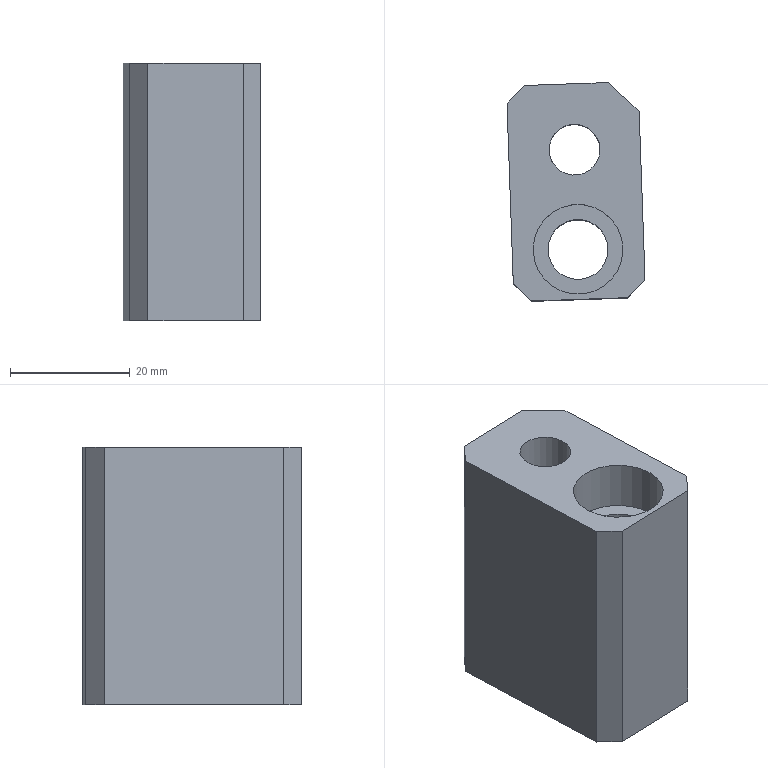Part | NX | features PH-10 2 | 1 solid | 16 faces | box 23.033 x 36.467 x 43 mm | volume 25123 mm3 | plane 12 | cylinder 4 | commonest cylinder face diameters 8.5 x1 10.001 x1 14.5 x1 15 x1
STEP:
#1=CARTESIAN_POINT('',(3339.766,-809.537,945.716));
#2=VERTEX_POINT('',#1);
#3=CARTESIAN_POINT('',(3332.266,-809.537,945.716));
#4=DIRECTION('',(0.,0.,1.));
#5=DIRECTION('',(1.,0.,0.));
#6=AXIS2_PLACEMENT_3D('',#3,#4,#5);
#7=CIRCLE('',#6,7.5);
#8=EDGE_CURVE('',#2,#2,#7,.F.);
#9=ORIENTED_EDGE('',*,*,#8,.T.);
#10=EDGE_LOOP('',(#9));
#11=FACE_BOUND('',#10,.T.);
#12=CARTESIAN_POINT('',(3335.932,-792.749,945.716));
#13=VERTEX_POINT('',#12);
#14=CARTESIAN_POINT('',(3331.685,-792.898,945.716));
#15=DIRECTION('',(0.,0.,1.));
#16=DIRECTION('',(0.9994,0.0349,0.));
#17=AXIS2_PLACEMENT_3D('',#14,#15,#16);
#18=CIRCLE('',#17,4.25);
#19=EDGE_CURVE('',#13,#13,#18,.T.);
#20=ORIENTED_EDGE('',*,*,#19,.F.);
#21=EDGE_LOOP('',(#20));
#22=FACE_BOUND('',#21,.T.);
#23=CARTESIAN_POINT('',(3342.469,-786.517,945.716));
#24=VERTEX_POINT('',#23);
#25=CARTESIAN_POINT('',(3343.446,-814.5,945.716));
#26=VERTEX_POINT('',#25);
#27=CARTESIAN_POINT('',(3342.922,-799.509,945.716));
#28=DIRECTION('',(0.0349,-0.9994,0.));
#29=VECTOR('',#28,1000.);
#30=LINE('',#27,#29);
#31=EDGE_CURVE('',#24,#26,#30,.T.);
#32=ORIENTED_EDGE('',*,*,#31,.F.);
#33=CARTESIAN_POINT('',(3337.297,-781.695,945.716));
#34=VERTEX_POINT('',#33);
#35=CARTESIAN_POINT('',(3343.503,-787.482,945.716));
#36=DIRECTION('',(0.7314,-0.682,0.));
#37=VECTOR('',#36,1000.);
#38=LINE('',#35,#37);
#39=EDGE_CURVE('',#24,#34,#38,.F.);
#40=ORIENTED_EDGE('',*,*,#39,.T.);
#41=CARTESIAN_POINT('',(3323.306,-782.183,945.716));
#42=VERTEX_POINT('',#41);
#43=CARTESIAN_POINT('',(3331.301,-781.904,945.716));
#44=DIRECTION('',(0.9994,0.0349,0.));
#45=VECTOR('',#44,1000.);
#46=LINE('',#43,#45);
#47=EDGE_CURVE('',#42,#34,#46,.T.);
#48=ORIENTED_EDGE('',*,*,#47,.F.);
#49=CARTESIAN_POINT('',(3320.412,-785.286,945.716));
#50=VERTEX_POINT('',#49);
#51=CARTESIAN_POINT('',(3318.483,-787.355,945.716));
#52=DIRECTION('',(0.682,0.7314,0.));
#53=VECTOR('',#52,1000.);
#54=LINE('',#51,#53);
#55=EDGE_CURVE('',#42,#50,#54,.F.);
#56=ORIENTED_EDGE('',*,*,#55,.T.);
#57=CARTESIAN_POINT('',(3321.459,-815.268,945.716));
#58=VERTEX_POINT('',#57);
#59=CARTESIAN_POINT('',(3320.936,-800.277,945.716));
#60=DIRECTION('',(-0.0349,0.9994,0.));
#61=VECTOR('',#60,1000.);
#62=LINE('',#59,#61);
#63=EDGE_CURVE('',#58,#50,#62,.T.);
#64=ORIENTED_EDGE('',*,*,#63,.F.);
#65=CARTESIAN_POINT('',(3324.562,-818.161,945.716));
#66=VERTEX_POINT('',#65);
#67=CARTESIAN_POINT('',(3319.39,-813.339,945.716));
#68=DIRECTION('',(-0.7314,0.682,0.));
#69=VECTOR('',#68,1000.);
#70=LINE('',#67,#69);
#71=EDGE_CURVE('',#58,#66,#70,.F.);
#72=ORIENTED_EDGE('',*,*,#71,.T.);
#73=CARTESIAN_POINT('',(3340.552,-817.603,945.716));
#74=VERTEX_POINT('',#73);
#75=CARTESIAN_POINT('',(3332.557,-817.882,945.716));
#76=DIRECTION('',(-0.9994,-0.0349,0.));
#77=VECTOR('',#76,1000.);
#78=LINE('',#75,#77);
#79=EDGE_CURVE('',#74,#66,#78,.T.);
#80=ORIENTED_EDGE('',*,*,#79,.F.);
#81=CARTESIAN_POINT('',(3345.375,-812.432,945.716));
#82=DIRECTION('',(-0.682,-0.7314,0.));
#83=VECTOR('',#82,1000.);
#84=LINE('',#81,#83);
#85=EDGE_CURVE('',#74,#26,#84,.F.);
#86=ORIENTED_EDGE('',*,*,#85,.T.);
#87=EDGE_LOOP('',(#32,#40,#48,#56,#64,#72,#80,#86));
#88=FACE_BOUND('',#87,.T.);
#89=CARTESIAN_POINT('',(3331.929,-799.893,945.716));
#90=DIRECTION('',(0.,0.,1.));
#91=DIRECTION('',(0.9994,0.0349,0.));
#92=AXIS2_PLACEMENT_3D('',#89,#90,#91);
#93=PLANE('',#92);
#94=ADVANCED_FACE('',(#11,#22,#88),#93,.T.);
#95=CARTESIAN_POINT('',(3324.562,-818.161,902.716));
#96=VERTEX_POINT('',#95);
#97=CARTESIAN_POINT('',(3340.552,-817.603,902.716));
#98=VERTEX_POINT('',#97);
#99=CARTESIAN_POINT('',(3332.557,-817.882,902.716));
#100=DIRECTION('',(0.9994,0.0349,0.));
#101=VECTOR('',#100,1000.);
#102=LINE('',#99,#101);
#103=EDGE_CURVE('',#96,#98,#102,.T.);
#104=ORIENTED_EDGE('',*,*,#103,.T.);
#105=CARTESIAN_POINT('',(3340.552,-817.603,920.716));
#106=DIRECTION('',(0.,0.,1.));
#107=VECTOR('',#106,1000.);
#108=LINE('',#105,#107);
#109=EDGE_CURVE('',#98,#74,#108,.T.);
#110=ORIENTED_EDGE('',*,*,#109,.T.);
#111=ORIENTED_EDGE('',*,*,#79,.T.);
#112=CARTESIAN_POINT('',(3324.562,-818.161,920.716));
#113=DIRECTION('',(0.,0.,-1.));
#114=VECTOR('',#113,1000.);
#115=LINE('',#112,#114);
#116=EDGE_CURVE('',#66,#96,#115,.T.);
#117=ORIENTED_EDGE('',*,*,#116,.T.);
#118=EDGE_LOOP('',(#104,#110,#111,#117));
#119=FACE_BOUND('',#118,.T.);
#120=CARTESIAN_POINT('',(3332.557,-817.882,920.716));
#121=DIRECTION('',(0.0349,-0.9994,0.));
#122=DIRECTION('',(0.,0.,-1.));
#123=AXIS2_PLACEMENT_3D('',#120,#121,#122);
#124=PLANE('',#123);
#125=ADVANCED_FACE('',(#119),#124,.T.);
#126=ORIENTED_EDGE('',*,*,#63,.T.);
#127=CARTESIAN_POINT('',(3320.412,-785.286,902.716));
#128=VERTEX_POINT('',#127);
#129=CARTESIAN_POINT('',(3320.412,-785.286,920.716));
#130=DIRECTION('',(0.,0.,-1.));
#131=VECTOR('',#130,1000.);
#132=LINE('',#129,#131);
#133=EDGE_CURVE('',#50,#128,#132,.T.);
#134=ORIENTED_EDGE('',*,*,#133,.T.);
#135=CARTESIAN_POINT('',(3321.459,-815.268,902.716));
#136=VERTEX_POINT('',#135);
#137=CARTESIAN_POINT('',(3320.936,-800.277,902.716));
#138=DIRECTION('',(0.0349,-0.9994,0.));
#139=VECTOR('',#138,1000.);
#140=LINE('',#137,#139);
#141=EDGE_CURVE('',#128,#136,#140,.T.);
#142=ORIENTED_EDGE('',*,*,#141,.T.);
#143=CARTESIAN_POINT('',(3321.459,-815.268,920.716));
#144=DIRECTION('',(0.,0.,1.));
#145=VECTOR('',#144,1000.);
#146=LINE('',#143,#145);
#147=EDGE_CURVE('',#136,#58,#146,.T.);
#148=ORIENTED_EDGE('',*,*,#147,.T.);
#149=EDGE_LOOP('',(#126,#134,#142,#148));
#150=FACE_BOUND('',#149,.T.);
#151=CARTESIAN_POINT('',(3320.936,-800.277,920.716));
#152=DIRECTION('',(-0.9994,-0.0349,0.));
#153=DIRECTION('',(0.,0.,1.));
#154=AXIS2_PLACEMENT_3D('',#151,#152,#153);
#155=PLANE('',#154);
#156=ADVANCED_FACE('',(#150),#155,.T.);
#157=ORIENTED_EDGE('',*,*,#47,.T.);
#158=CARTESIAN_POINT('',(3337.297,-781.695,902.716));
#159=VERTEX_POINT('',#158);
#160=CARTESIAN_POINT('',(3337.297,-781.695,920.716));
#161=DIRECTION('',(0.,0.,-1.));
#162=VECTOR('',#161,1000.);
#163=LINE('',#160,#162);
#164=EDGE_CURVE('',#34,#159,#163,.T.);
#165=ORIENTED_EDGE('',*,*,#164,.T.);
#166=CARTESIAN_POINT('',(3323.306,-782.183,902.716));
#167=VERTEX_POINT('',#166);
#168=CARTESIAN_POINT('',(3331.301,-781.904,902.716));
#169=DIRECTION('',(-0.9994,-0.0349,0.));
#170=VECTOR('',#169,1000.);
#171=LINE('',#168,#170);
#172=EDGE_CURVE('',#159,#167,#171,.T.);
#173=ORIENTED_EDGE('',*,*,#172,.T.);
#174=CARTESIAN_POINT('',(3323.306,-782.183,920.716));
#175=DIRECTION('',(0.,0.,1.));
#176=VECTOR('',#175,1000.);
#177=LINE('',#174,#176);
#178=EDGE_CURVE('',#167,#42,#177,.T.);
#179=ORIENTED_EDGE('',*,*,#178,.T.);
#180=EDGE_LOOP('',(#157,#165,#173,#179));
#181=FACE_BOUND('',#180,.T.);
#182=CARTESIAN_POINT('',(3331.301,-781.904,920.716));
#183=DIRECTION('',(-0.0349,0.9994,0.));
#184=DIRECTION('',(0.,0.,1.));
#185=AXIS2_PLACEMENT_3D('',#182,#183,#184);
#186=PLANE('',#185);
#187=ADVANCED_FACE('',(#181),#186,.T.);
#188=CARTESIAN_POINT('',(3327.265,-809.537,902.716));
#189=VERTEX_POINT('',#188);
#190=CARTESIAN_POINT('',(3332.266,-809.537,902.716));
#191=DIRECTION('',(0.,0.,-1.));
#192=DIRECTION('',(-1.,0.,0.));
#193=AXIS2_PLACEMENT_3D('',#190,#191,#192);
#194=CIRCLE('',#193,5.);
#195=EDGE_CURVE('',#189,#189,#194,.T.);
#196=ORIENTED_EDGE('',*,*,#195,.F.);
#197=EDGE_LOOP('',(#196));
#198=FACE_BOUND('',#197,.T.);
#199=CARTESIAN_POINT('',(3324.435,-792.898,902.716));
#200=VERTEX_POINT('',#199);
#201=CARTESIAN_POINT('',(3331.685,-792.898,902.716));
#202=DIRECTION('',(0.,0.,-1.));
#203=DIRECTION('',(-1.,0.,0.));
#204=AXIS2_PLACEMENT_3D('',#201,#202,#203);
#205=CIRCLE('',#204,7.25);
#206=EDGE_CURVE('',#200,#200,#205,.F.);
#207=ORIENTED_EDGE('',*,*,#206,.T.);
#208=EDGE_LOOP('',(#207));
#209=FACE_BOUND('',#208,.T.);
#210=ORIENTED_EDGE('',*,*,#172,.F.);
#211=CARTESIAN_POINT('',(3342.469,-786.517,902.716));
#212=VERTEX_POINT('',#211);
#213=CARTESIAN_POINT('',(3343.503,-787.482,902.716));
#214=DIRECTION('',(-0.7314,0.682,0.));
#215=VECTOR('',#214,1000.);
#216=LINE('',#213,#215);
#217=EDGE_CURVE('',#159,#212,#216,.F.);
#218=ORIENTED_EDGE('',*,*,#217,.T.);
#219=CARTESIAN_POINT('',(3343.446,-814.5,902.716));
#220=VERTEX_POINT('',#219);
#221=CARTESIAN_POINT('',(3342.922,-799.509,902.716));
#222=DIRECTION('',(-0.0349,0.9994,0.));
#223=VECTOR('',#222,1000.);
#224=LINE('',#221,#223);
#225=EDGE_CURVE('',#220,#212,#224,.T.);
#226=ORIENTED_EDGE('',*,*,#225,.F.);
#227=CARTESIAN_POINT('',(3345.375,-812.432,902.716));
#228=DIRECTION('',(0.682,0.7314,0.));
#229=VECTOR('',#228,1000.);
#230=LINE('',#227,#229);
#231=EDGE_CURVE('',#220,#98,#230,.F.);
#232=ORIENTED_EDGE('',*,*,#231,.T.);
#233=ORIENTED_EDGE('',*,*,#103,.F.);
#234=CARTESIAN_POINT('',(3319.39,-813.339,902.716));
#235=DIRECTION('',(0.7314,-0.682,0.));
#236=VECTOR('',#235,1000.);
#237=LINE('',#234,#236);
#238=EDGE_CURVE('',#96,#136,#237,.F.);
#239=ORIENTED_EDGE('',*,*,#238,.T.);
#240=ORIENTED_EDGE('',*,*,#141,.F.);
#241=CARTESIAN_POINT('',(3318.483,-787.355,902.716));
#242=DIRECTION('',(-0.682,-0.7314,0.));
#243=VECTOR('',#242,1000.);
#244=LINE('',#241,#243);
#245=EDGE_CURVE('',#128,#167,#244,.F.);
#246=ORIENTED_EDGE('',*,*,#245,.T.);
#247=EDGE_LOOP('',(#210,#218,#226,#232,#233,#239,#240,#246));
#248=FACE_BOUND('',#247,.T.);
#249=CARTESIAN_POINT('',(3331.929,-799.893,902.716));
#250=DIRECTION('',(0.,0.,-1.));
#251=DIRECTION('',(-0.9994,-0.0349,0.));
#252=AXIS2_PLACEMENT_3D('',#249,#250,#251);
#253=PLANE('',#252);
#254=ADVANCED_FACE('',(#198,#209,#248),#253,.T.);
#255=ORIENTED_EDGE('',*,*,#225,.T.);
#256=CARTESIAN_POINT('',(3342.469,-786.517,920.716));
#257=DIRECTION('',(0.,0.,1.));
#258=VECTOR('',#257,1000.);
#259=LINE('',#256,#258);
#260=EDGE_CURVE('',#212,#24,#259,.T.);
#261=ORIENTED_EDGE('',*,*,#260,.T.);
#262=ORIENTED_EDGE('',*,*,#31,.T.);
#263=CARTESIAN_POINT('',(3343.446,-814.5,920.716));
#264=DIRECTION('',(0.,0.,-1.));
#265=VECTOR('',#264,1000.);
#266=LINE('',#263,#265);
#267=EDGE_CURVE('',#26,#220,#266,.T.);
#268=ORIENTED_EDGE('',*,*,#267,.T.);
#269=EDGE_LOOP('',(#255,#261,#262,#268));
#270=FACE_BOUND('',#269,.T.);
#271=CARTESIAN_POINT('',(3342.922,-799.509,920.716));
#272=DIRECTION('',(0.9994,0.0349,0.));
#273=DIRECTION('',(0.,0.,-1.));
#274=AXIS2_PLACEMENT_3D('',#271,#272,#273);
#275=PLANE('',#274);
#276=ADVANCED_FACE('',(#270),#275,.T.);
#277=ORIENTED_EDGE('',*,*,#231,.F.);
#278=ORIENTED_EDGE('',*,*,#267,.F.);
#279=ORIENTED_EDGE('',*,*,#85,.F.);
#280=ORIENTED_EDGE('',*,*,#109,.F.);
#281=EDGE_LOOP('',(#277,#278,#279,#280));
#282=FACE_BOUND('',#281,.T.);
#283=CARTESIAN_POINT('',(3340.552,-817.603,920.716));
#284=DIRECTION('',(-0.7314,0.682,0.));
#285=DIRECTION('',(-0.682,-0.7314,0.));
#286=AXIS2_PLACEMENT_3D('',#283,#284,#285);
#287=PLANE('',#286);
#288=ADVANCED_FACE('',(#282),#287,.F.);
#289=ORIENTED_EDGE('',*,*,#238,.F.);
#290=ORIENTED_EDGE('',*,*,#116,.F.);
#291=ORIENTED_EDGE('',*,*,#71,.F.);
#292=ORIENTED_EDGE('',*,*,#147,.F.);
#293=EDGE_LOOP('',(#289,#290,#291,#292));
#294=FACE_BOUND('',#293,.T.);
#295=CARTESIAN_POINT('',(3321.459,-815.268,920.716));
#296=DIRECTION('',(0.682,0.7314,0.));
#297=DIRECTION('',(-0.7314,0.682,0.));
#298=AXIS2_PLACEMENT_3D('',#295,#296,#297);
#299=PLANE('',#298);
#300=ADVANCED_FACE('',(#294),#299,.F.);
#301=ORIENTED_EDGE('',*,*,#245,.F.);
#302=ORIENTED_EDGE('',*,*,#133,.F.);
#303=ORIENTED_EDGE('',*,*,#55,.F.);
#304=ORIENTED_EDGE('',*,*,#178,.F.);
#305=EDGE_LOOP('',(#301,#302,#303,#304));
#306=FACE_BOUND('',#305,.T.);
#307=CARTESIAN_POINT('',(3323.306,-782.183,920.716));
#308=DIRECTION('',(0.7314,-0.682,0.));
#309=DIRECTION('',(0.682,0.7314,0.));
#310=AXIS2_PLACEMENT_3D('',#307,#308,#309);
#311=PLANE('',#310);
#312=ADVANCED_FACE('',(#306),#311,.F.);
#313=CARTESIAN_POINT('',(3335.935,-792.898,913.716));
#314=VERTEX_POINT('',#313);
#315=CARTESIAN_POINT('',(3331.685,-792.898,913.716));
#316=DIRECTION('',(0.,0.,1.));
#317=DIRECTION('',(1.,0.,0.));
#318=AXIS2_PLACEMENT_3D('',#315,#316,#317);
#319=CIRCLE('',#318,4.25);
#320=EDGE_CURVE('',#314,#314,#319,.T.);
#321=ORIENTED_EDGE('',*,*,#320,.T.);
#322=EDGE_LOOP('',(#321));
#323=FACE_BOUND('',#322,.T.);
#324=CARTESIAN_POINT('',(3338.935,-792.898,913.716));
#325=VERTEX_POINT('',#324);
#326=CARTESIAN_POINT('',(3331.685,-792.898,913.716));
#327=DIRECTION('',(0.,0.,1.));
#328=DIRECTION('',(1.,0.,0.));
#329=AXIS2_PLACEMENT_3D('',#326,#327,#328);
#330=CIRCLE('',#329,7.25);
#331=EDGE_CURVE('',#325,#325,#330,.T.);
#332=ORIENTED_EDGE('',*,*,#331,.F.);
#333=EDGE_LOOP('',(#332));
#334=FACE_BOUND('',#333,.T.);
#335=CARTESIAN_POINT('',(3331.685,-792.898,913.716));
#336=DIRECTION('',(0.,0.,1.));
#337=DIRECTION('',(0.9994,0.0349,0.));
#338=AXIS2_PLACEMENT_3D('',#335,#336,#337);
#339=PLANE('',#338);
#340=ADVANCED_FACE('',(#323,#334),#339,.F.);
#341=ORIENTED_EDGE('',*,*,#206,.F.);
#342=EDGE_LOOP('',(#341));
#343=FACE_BOUND('',#342,.T.);
#344=ORIENTED_EDGE('',*,*,#331,.T.);
#345=EDGE_LOOP('',(#344));
#346=FACE_BOUND('',#345,.T.);
#347=CARTESIAN_POINT('',(3331.685,-792.898,931.716));
#348=DIRECTION('',(0.,0.,-1.));
#349=DIRECTION('',(0.9994,0.0349,0.));
#350=AXIS2_PLACEMENT_3D('',#347,#348,#349);
#351=CYLINDRICAL_SURFACE('',#350,7.25);
#352=ADVANCED_FACE('',(#343,#346),#351,.F.);
#353=ORIENTED_EDGE('',*,*,#19,.T.);
#354=EDGE_LOOP('',(#353));
#355=FACE_BOUND('',#354,.T.);
#356=ORIENTED_EDGE('',*,*,#320,.F.);
#357=EDGE_LOOP('',(#356));
#358=FACE_BOUND('',#357,.T.);
#359=CARTESIAN_POINT('',(3331.685,-792.898,946.716));
#360=DIRECTION('',(0.,0.,-1.));
#361=DIRECTION('',(0.9994,0.0349,0.));
#362=AXIS2_PLACEMENT_3D('',#359,#360,#361);
#363=CYLINDRICAL_SURFACE('',#362,4.25);
#364=ADVANCED_FACE('',(#355,#358),#363,.F.);
#365=ORIENTED_EDGE('',*,*,#195,.T.);
#366=EDGE_LOOP('',(#365));
#367=FACE_BOUND('',#366,.T.);
#368=CARTESIAN_POINT('',(3327.265,-809.537,937.516));
#369=VERTEX_POINT('',#368);
#370=CARTESIAN_POINT('',(3332.266,-809.537,937.516));
#371=DIRECTION('',(0.,0.,-1.));
#372=DIRECTION('',(-1.,0.,0.));
#373=AXIS2_PLACEMENT_3D('',#370,#371,#372);
#374=CIRCLE('',#373,5.);
#375=EDGE_CURVE('',#369,#369,#374,.T.);
#376=ORIENTED_EDGE('',*,*,#375,.F.);
#377=EDGE_LOOP('',(#376));
#378=FACE_BOUND('',#377,.T.);
#379=CARTESIAN_POINT('',(3332.266,-809.537,945.716));
#380=DIRECTION('',(0.,0.,-1.));
#381=DIRECTION('',(1.,0.,0.));
#382=AXIS2_PLACEMENT_3D('',#379,#380,#381);
#383=CYLINDRICAL_SURFACE('',#382,5.);
#384=ADVANCED_FACE('',(#367,#378),#383,.F.);
#385=ORIENTED_EDGE('',*,*,#375,.T.);
#386=EDGE_LOOP('',(#385));
#387=FACE_BOUND('',#386,.T.);
#388=CARTESIAN_POINT('',(3324.766,-809.537,937.516));
#389=VERTEX_POINT('',#388);
#390=CARTESIAN_POINT('',(3332.266,-809.537,937.516));
#391=DIRECTION('',(0.,0.,-1.));
#392=DIRECTION('',(-1.,0.,0.));
#393=AXIS2_PLACEMENT_3D('',#390,#391,#392);
#394=CIRCLE('',#393,7.5);
#395=EDGE_CURVE('',#389,#389,#394,.T.);
#396=ORIENTED_EDGE('',*,*,#395,.F.);
#397=EDGE_LOOP('',(#396));
#398=FACE_BOUND('',#397,.T.);
#399=CARTESIAN_POINT('',(3332.266,-809.537,937.516));
#400=DIRECTION('',(0.,0.,-1.));
#401=DIRECTION('',(-1.,0.,0.));
#402=AXIS2_PLACEMENT_3D('',#399,#400,#401);
#403=PLANE('',#402);
#404=ADVANCED_FACE('',(#387,#398),#403,.F.);
#405=ORIENTED_EDGE('',*,*,#395,.T.);
#406=EDGE_LOOP('',(#405));
#407=FACE_BOUND('',#406,.T.);
#408=ORIENTED_EDGE('',*,*,#8,.F.);
#409=EDGE_LOOP('',(#408));
#410=FACE_BOUND('',#409,.T.);
#411=CARTESIAN_POINT('',(3332.266,-809.537,945.716));
#412=DIRECTION('',(0.,0.,-1.));
#413=DIRECTION('',(1.,0.,0.));
#414=AXIS2_PLACEMENT_3D('',#411,#412,#413);
#415=CYLINDRICAL_SURFACE('',#414,7.5);
#416=ADVANCED_FACE('',(#407,#410),#415,.F.);
#417=ORIENTED_EDGE('',*,*,#39,.F.);
#418=ORIENTED_EDGE('',*,*,#260,.F.);
#419=ORIENTED_EDGE('',*,*,#217,.F.);
#420=ORIENTED_EDGE('',*,*,#164,.F.);
#421=EDGE_LOOP('',(#417,#418,#419,#420));
#422=FACE_BOUND('',#421,.T.);
#423=CARTESIAN_POINT('',(3337.297,-781.695,920.716));
#424=DIRECTION('',(-0.682,-0.7314,0.));
#425=DIRECTION('',(0.,0.,-1.));
#426=AXIS2_PLACEMENT_3D('',#423,#424,#425);
#427=PLANE('',#426);
#428=ADVANCED_FACE('',(#422),#427,.F.);
#429=CLOSED_SHELL('',(#94,#125,#156,#187,#254,#276,#288,#300,#312,#340,#352,#364,#384,#404,#416,#428));
#430=MANIFOLD_SOLID_BREP('',#429);
#431=(LENGTH_UNIT()NAMED_UNIT(*)SI_UNIT(.MILLI.,.METRE.));
#432=UNCERTAINTY_MEASURE_WITH_UNIT(LENGTH_MEASURE(0.00001),#431,'','');
#433=(NAMED_UNIT(*)PLANE_ANGLE_UNIT()SI_UNIT($,.RADIAN.));
#434=(NAMED_UNIT(*)SI_UNIT($,.STERADIAN.)SOLID_ANGLE_UNIT());
#435=(GEOMETRIC_REPRESENTATION_CONTEXT(3)GLOBAL_UNCERTAINTY_ASSIGNED_CONTEXT((#432))GLOBAL_UNIT_ASSIGNED_CONTEXT((#431,#433,#434))REPRESENTATION_CONTEXT('',''));
#436=ADVANCED_BREP_SHAPE_REPRESENTATION('',(#430),#435);